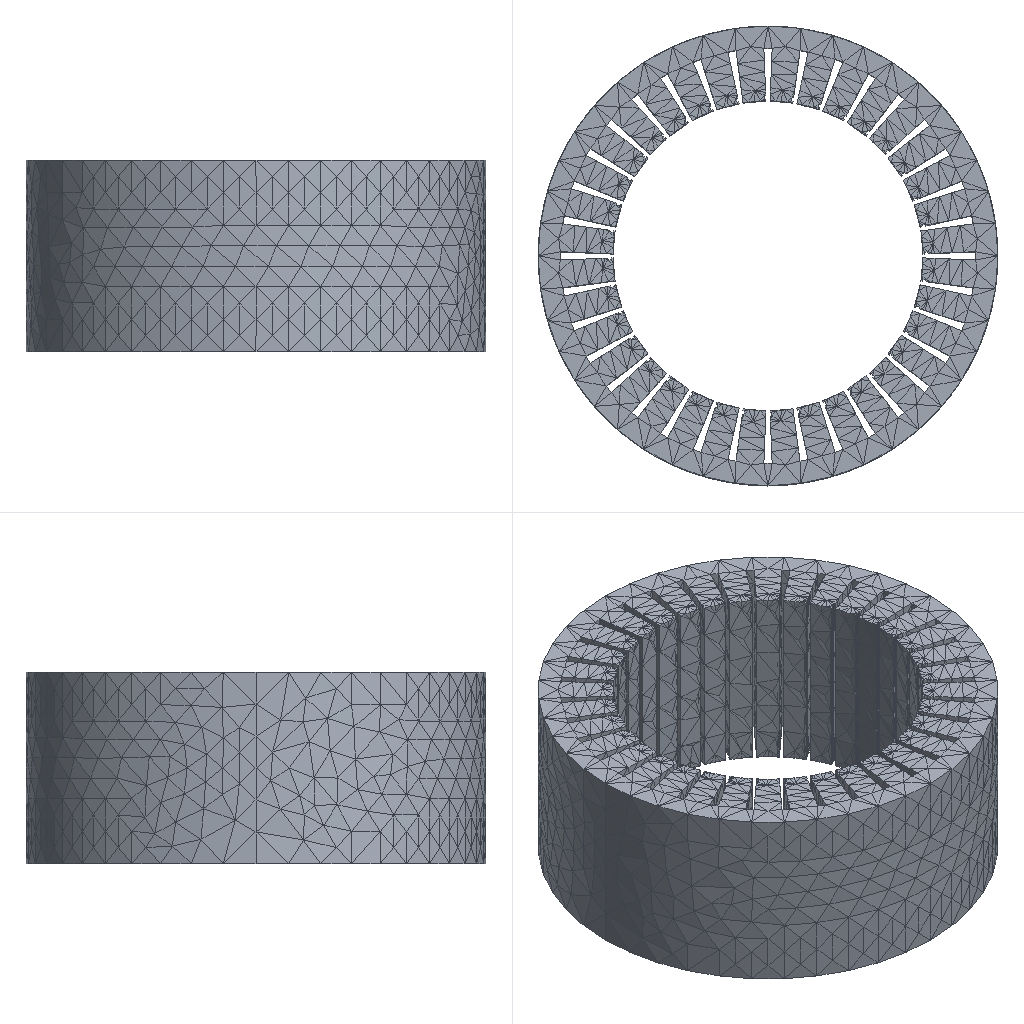Simulation study | ansys workbench
Set-up summary:
category,name,step,type,value,unit,region
solver,ansys_mapdl
solver,version,,,22.1
units,MPA,,stated
analysis,deck,,modal,modal
load_step,requested,,,1
analysis,nlgeom,,,False
mesh,nodes,,,30832
mesh,elements,,,16223
element_type,ANSYS 187 (type 1),,solid,16223
load,load commands in deck,,count,0
bc,support commands in deck,,count,0
material,1,,in results
check,setup vs results,,match
Ansys APDL input file, long lists of numbers shortened:
/batch
/config,noeldb,1     ! force off writing results to database
*get,_wallstrt,active,,time,wall
! ANSYS input file written by Workbench version 2022 R1
! File used for geometry attach: F:\ansys（分析文件汇总)\定子铁芯有限元分析\定子铁芯.STEP
/title,wbnew--__ (B5)
! ****** Begin Custom Load Command Snippet ******
/COM, ACT Extensions:
/COM,     LSDYNA, 2021.1
/COM,
! ****** End   Custom Load Command Snippet ******
*DIM,_wb_ProjectScratch_dir,string,248
_wb_ProjectScratch_dir(1) = 'C:\Users\Administrator\AppData\Local\Temp\WB_Administrator_1504_2\_ProjectScratch\Scr7F7D\'
*DIM,_wb_SolverFiles_dir,string,248
_wb_SolverFiles_dir(1) = 'C:\Users\Administrator\AppData\Local\Temp\WB_Administrator_1504_2\wbnew_files\dp0\SYS\MECH\'
*DIM,_wb_userfiles_dir,string,248
_wb_userfiles_dir(1) = 'C:\Users\Administrator\AppData\Local\Temp\WB_Administrator_1504_2\wbnew_files\user_files\'
/com,--- Data in consistent NMM units. See Solving Units in the help system for more information.
/units,MPA
/nopr
/wb,file,start              !  signify a WB generated input file
/prep7
! Turn off shape checking because checks already performed inside WB mesher.
! See help system for more information.
SHPP,OFF,,NOWARN
/nolist
etcon,set             ! allow ANSYS to choose best KEYOP's for 180x elements, resets any applicable keyopt to MAPDL defaults
/com,*********** Nodes for the whole assembly ***********
nblock,3,,33915
(1i9,3e20.9e3)
        1     3.055000000E+02     3.741295971E-14     2.550000000E+02
! (30831 more lines like these left out)
-1
/wb,elem,start            !  set before creation of elements
/com,*********** Elements for Body 1 "____-FreeParts|__(__)1" ***********
et,1,187
eblock,19,solid,,16223
(19i9)
        1        1        1        1        0        0        0        0       10        0        1     2996     3834     4713     4577    24398    28311    24403    24402
! (32445 more lines like these left out)
-1
/wb,elem,end               !  done creating elements
/com,*********** Send User Defined Coordinate System(s) ***********
csys,0
toffst,273.15,  ! Temperature offset from absolute zero
/com,*********** Set Reference Temperature ***********
tref,22.
/wb,mat,start              !  starting to send materials
/com,*********** Send Materials ***********
Temperature = 'TEMP' ! Temperature
MP,DENS,1,7.85e-09,	! tonne mm^-3
MP,ALPX,1,1.2e-05,	! C^-1
MP,C,1,434000000,	! mm^2 s^-2 C^-1
MP,KXX,1,60.5,	! tonne mm s^-3 C^-1
MP,RSVX,1,0.00017,	! ohm mm
MP,EX,1,200000,	! tonne s^-2 mm^-1
MP,NUXY,1,0.3,
MP,MURX,1,10000,
/wb,mat,end                !  done sending materials
!************************* Model Summary ********************
!____-FreeParts|__(__)1,	结构钢,	matid,	1
!************************* End Model Summary ********************
! get the diagonal of the bounding box. Needed later for other things
*get,_xmin,node,,mnloc,x
*get,_ymin,node,,mnloc,y
*get,_zmin,node,,mnloc,z
*get,_xmax,node,,mxloc,x
*get,_ymax,node,,mxloc,y
*get,_zmax,node,,mxloc,z
_ASMDIAG=(_xmax-_xmin)*(_xmax-_xmin)+(_ymax-_ymin)*(_ymax-_ymin)+(_zmax-_zmin)*(_zmax-_zmin)
_ASMDIAG=SQRT(_ASMDIAG)
/wb,contact,start          !  starting to send contact
/wb,contact,end            !  done creating contacts
/golist
/wb,load,start             !  starting to send loads
/gst,on,on
fini
*get,_numnode,node,0,count
*get,_numelem,elem,0,count
*get, _MAXELEMNUM, elem, 0, NUM, MAX
*get, _MAXNODENUM, node, 0, NUM, MAX
*get, _MAXELEMTYPE, etyp, 0, NUM, MAX
*get, _MAXREALCONST, real, 0, NUM, MAX
/go
/wb,load,end               !  done creating loads
/com,--- Number of total nodes = %_numnode%
/com,--- Number of contact elements = 0
/com,--- Number of spring elements = 0
/com,--- Number of bearing elements = 0
/com,--- Number of solid elements = 16223
/com,--- Number of condensed parts = 0
/com,--- Number of total elements = %_numelem%
*get,_wallbsol,active,,time,wall
/solu
antype,2                   ! modal analysis
_thickRatio=  0     ! Ratio of thick parts in the model
modopt,lanb,20
outres,erase
outres,all,none
outres,nsol,all
outres,etmp,all
mxpand                    ! default expand in case of complex solution
dmpopt,esav,no
dmpopt,emat,no
dmpopt,full,no
! *********** WB SOLVE COMMAND ***********
! check interactive state
*get,ANSINTER_,active,,int
*if,ANSINTER_,ne,0,then
/eof
*endif
solve
/com *************** Write FE CONNECTORS *********
CEWRITE,file,ce,,INTE
*get,_nmodalsolproc,active,0,numcpu
fini
/nopr
*get,_numnode,node,0,count
*get,_numelem,elem,0,count
*get, _MAXELEMNUM, elem, 0, NUM, MAX
*get, _MAXNODENUM, node, 0, NUM, MAX,,,INTERNAL
*get, _MAXELEMTYPE, etyp, 0, NUM, MAX
*get, _MAXREALCONST, real, 0, NUM, MAX
/gopr
*get,_wallasol,active,,time,wall
/post1
/nopr
*dim,_direction,CHAR,6,1
_direction(1) = 'X'
_direction(2) = 'Y'
_direction(3) = 'Z'
_direction(4) = 'ROTX'
_direction(5) = 'ROTY'
_direction(6) = 'ROTZ'
*get,_lastLS,active,0,set,LSTP
*get,_beginset,active,0,set,nset,first,_lastLS
*get,_endset,active,0,set,nset,last,_lastLS
_nummodes = 0
*if,_endset,gt,0,then
_nummodes = _endset - _beginset + 1
*endif
*do,i_mode,1,_nummodes
   *do,j_component,1,6
			*get,PFACT_%i_mode%_%j_component%,MODE,%i_mode%,PFACT,,DIREC,_direction(%j_component%)
   *enddo
*enddo
*dim,_tmdirection,CHAR,6,1
_tmdirection(1) = 'X'
_tmdirection(2) = 'Y'
_tmdirection(3) = 'Z'
_tmdirection(4) = 'X'
_tmdirection(5) = 'Y'
_tmdirection(6) = 'Z'
*do,j_component,1,6
    *if,j_component,gt,3,then
        *get,TOTALMASS_%j_component%,ELEM,0,IOR,_tmdirection(%j_component%)
    *else
        *get,TOTALMASS_%j_component%,ELEM,0,MTOT,_tmdirection(%j_component%)
    *endif
*enddo
/gopr
xmlo,ENCODING,ISO-8859-1
xmlo,parm
/xml,parm,xml
fini
/gopr
*get,_walldone,active,,time,wall
_preptime=(_wallbsol-_wallstrt)*3600
_solvtime=(_wallasol-_wallbsol)*3600
_posttime=(_walldone-_wallasol)*3600
_totaltim=(_walldone-_wallstrt)*3600
*get,_dlbratio,active,0,solu,dlbr
*get,_combtime,active,0,solu,comb
*get,_ssmode,active,0,solu,ssmm
*get,_ndofs,active,0,solu,ndof
/fclean				!clean distributed files
/com,--- Total number of nodes = %_numnode%
/com,--- Total number of elements = %_numelem%
/com,--- Element load balance ratio = %_dlbratio%
/com,--- Time to combine distributed files = %_combtime%
/com,--- Sparse memory mode = %_ssmode%
/com,--- Number of DOF = %_ndofs%
/wb,file,end               ! done with WB generated input
Results summary:
result,analysis,,,modal
result,last_loadstep,,,1
result,primary field,,,displacement